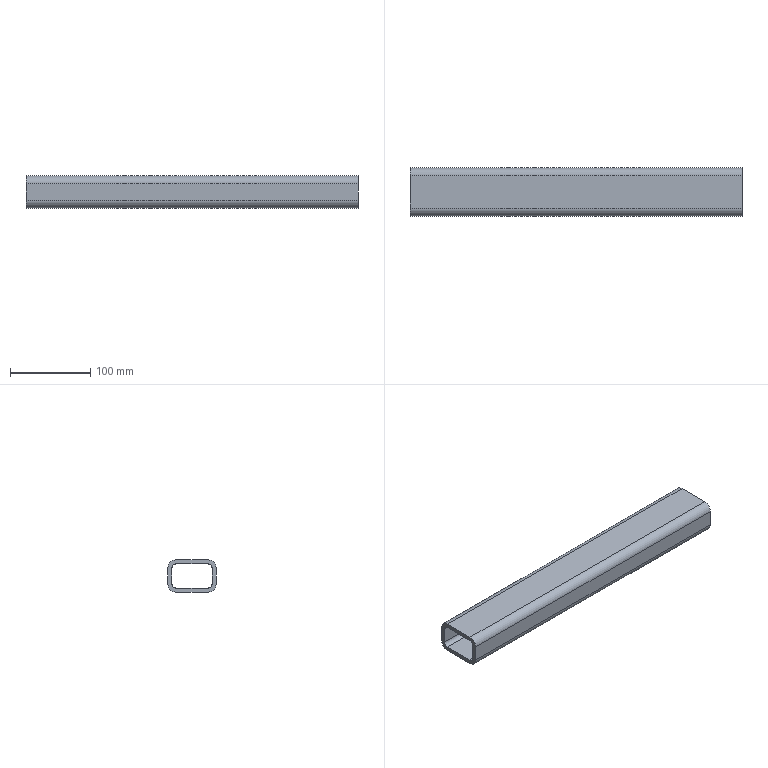Part | STEP file | HL4GD-1.30.112 base frame support longitudinal beam--20251212 | 1 solid | 18 faces | box 414 x 60 x 40 mm | volume 345946 mm3 | plane 10 | cylinder 8 | commonest cylinder face diameters 10 x4 20 x4
STEP:
#1=CARTESIAN_POINT('',(0.,0.,0.));
#2=DIRECTION('',(0.,0.,1.));
#3=DIRECTION('',(1.,0.,0.));
#4=AXIS2_PLACEMENT_3D('',#1,#2,#3);
#5=CARTESIAN_POINT('',(2009.,540.,400.));
#6=VERTEX_POINT('',#5);
#7=CARTESIAN_POINT('',(2009.,535.,395.));
#8=VERTEX_POINT('',#7);
#9=CARTESIAN_POINT('',(2009.,540.,395.));
#10=DIRECTION('',(1.,0.,0.));
#11=DIRECTION('',(0.,0.,-1.));
#12=AXIS2_PLACEMENT_3D('',#9,#10,#11);
#13=CIRCLE('',#12,5.);
#14=CARTESIAN_POINT('',(2555.,540.,395.));
#15=DIRECTION('',(1.,0.,0.));
#16=DIRECTION('',(0.,0.,1.));
#17=AXIS2_PLACEMENT_3D('',#14,#15,#16);
#18=CYLINDRICAL_SURFACE('',#17,5.);
#19=CARTESIAN_POINT('',(-3.142,-546.));
#20=DIRECTION('',(1.,0.));
#21=VECTOR('',#20,1.);
#22=LINE('',#19,#21);
#23=(GEOMETRIC_REPRESENTATION_CONTEXT(2)PARAMETRIC_REPRESENTATION_CONTEXT()REPRESENTATION_CONTEXT('',''));
#24=DEFINITIONAL_REPRESENTATION('',(#22),#23);
#25=PCURVE('',#18,#24);
#26=CARTESIAN_POINT('',(2009.,590.,375.));
#27=DIRECTION('',(1.,0.,0.));
#28=DIRECTION('',(0.,0.,-1.));
#29=AXIS2_PLACEMENT_3D('',#26,#27,#28);
#30=PLANE('',#29);
#31=CARTESIAN_POINT('',(-20.,-50.));
#32=DIRECTION('',(1.,0.));
#33=AXIS2_PLACEMENT_2D('',#31,#32);
#34=CIRCLE('',#33,5.);
#35=(GEOMETRIC_REPRESENTATION_CONTEXT(2)PARAMETRIC_REPRESENTATION_CONTEXT()REPRESENTATION_CONTEXT('',''));
#36=DEFINITIONAL_REPRESENTATION('',(#34),#35);
#37=PCURVE('',#30,#36);
#38=SURFACE_CURVE('',#13,(#25,#37),.PCURVE_S1.);
#39=EDGE_CURVE('',#6,#8,#38,.T.);
#40=ORIENTED_EDGE('',*,*,#39,.F.);
#41=CARTESIAN_POINT('',(1595.,540.,400.));
#42=VERTEX_POINT('',#41);
#43=CARTESIAN_POINT('',(2555.,540.,400.));
#44=DIRECTION('',(-1.,0.,0.));
#45=VECTOR('',#44,1.);
#46=LINE('',#43,#45);
#47=CARTESIAN_POINT('',(0.,0.));
#48=DIRECTION('',(0.,-1.));
#49=VECTOR('',#48,1.);
#50=LINE('',#47,#49);
#51=(GEOMETRIC_REPRESENTATION_CONTEXT(2)PARAMETRIC_REPRESENTATION_CONTEXT()REPRESENTATION_CONTEXT('',''));
#52=DEFINITIONAL_REPRESENTATION('',(#50),#51);
#53=PCURVE('',#18,#52);
#54=CARTESIAN_POINT('',(2555.,540.,400.));
#55=DIRECTION('',(0.,0.,-1.));
#56=DIRECTION('',(0.,-1.,0.));
#57=AXIS2_PLACEMENT_3D('',#54,#55,#56);
#58=PLANE('',#57);
#59=CARTESIAN_POINT('',(0.,0.));
#60=DIRECTION('',(0.,1.));
#61=VECTOR('',#60,1.);
#62=LINE('',#59,#61);
#63=(GEOMETRIC_REPRESENTATION_CONTEXT(2)PARAMETRIC_REPRESENTATION_CONTEXT()REPRESENTATION_CONTEXT('',''));
#64=DEFINITIONAL_REPRESENTATION('',(#62),#63);
#65=PCURVE('',#58,#64);
#66=SURFACE_CURVE('',#46,(#53,#65),.PCURVE_S1.);
#67=EDGE_CURVE('',#6,#42,#66,.T.);
#68=ORIENTED_EDGE('',*,*,#67,.T.);
#69=CARTESIAN_POINT('',(1595.,535.,395.));
#70=VERTEX_POINT('',#69);
#71=CARTESIAN_POINT('',(1595.,540.,395.));
#72=DIRECTION('',(1.,0.,0.));
#73=DIRECTION('',(0.,0.,1.));
#74=AXIS2_PLACEMENT_3D('',#71,#72,#73);
#75=CIRCLE('',#74,5.);
#76=CARTESIAN_POINT('',(0.,-960.));
#77=DIRECTION('',(1.,0.));
#78=VECTOR('',#77,1.);
#79=LINE('',#76,#78);
#80=(GEOMETRIC_REPRESENTATION_CONTEXT(2)PARAMETRIC_REPRESENTATION_CONTEXT()REPRESENTATION_CONTEXT('',''));
#81=DEFINITIONAL_REPRESENTATION('',(#79),#80);
#82=PCURVE('',#18,#81);
#83=CARTESIAN_POINT('',(1595.,406.07,581.07));
#84=DIRECTION('',(1.,0.,0.));
#85=DIRECTION('',(0.,0.,1.));
#86=AXIS2_PLACEMENT_3D('',#83,#84,#85);
#87=PLANE('',#86);
#88=CARTESIAN_POINT('',(-186.07,-133.93));
#89=DIRECTION('',(1.,0.));
#90=AXIS2_PLACEMENT_2D('',#88,#89);
#91=CIRCLE('',#90,5.);
#92=(GEOMETRIC_REPRESENTATION_CONTEXT(2)PARAMETRIC_REPRESENTATION_CONTEXT()REPRESENTATION_CONTEXT('',''));
#93=DEFINITIONAL_REPRESENTATION('',(#91),#92);
#94=PCURVE('',#87,#93);
#95=SURFACE_CURVE('',#75,(#82,#94),.PCURVE_S1.);
#96=EDGE_CURVE('',#42,#70,#95,.T.);
#97=ORIENTED_EDGE('',*,*,#96,.T.);
#98=CARTESIAN_POINT('',(2555.,535.,395.));
#99=DIRECTION('',(-1.,0.,0.));
#100=VECTOR('',#99,1.);
#101=LINE('',#98,#100);
#102=CARTESIAN_POINT('',(1.571,0.));
#103=DIRECTION('',(0.,-1.));
#104=VECTOR('',#103,1.);
#105=LINE('',#102,#104);
#106=(GEOMETRIC_REPRESENTATION_CONTEXT(2)PARAMETRIC_REPRESENTATION_CONTEXT()REPRESENTATION_CONTEXT('',''));
#107=DEFINITIONAL_REPRESENTATION('',(#105),#106);
#108=PCURVE('',#18,#107);
#109=CARTESIAN_POINT('',(2555.,535.,375.));
#110=DIRECTION('',(0.,1.,0.));
#111=DIRECTION('',(0.,0.,-1.));
#112=AXIS2_PLACEMENT_3D('',#109,#110,#111);
#113=PLANE('',#112);
#114=CARTESIAN_POINT('',(-20.,0.));
#115=DIRECTION('',(0.,1.));
#116=VECTOR('',#115,1.);
#117=LINE('',#114,#116);
#118=(GEOMETRIC_REPRESENTATION_CONTEXT(2)PARAMETRIC_REPRESENTATION_CONTEXT()REPRESENTATION_CONTEXT('',''));
#119=DEFINITIONAL_REPRESENTATION('',(#117),#118);
#120=PCURVE('',#113,#119);
#121=SURFACE_CURVE('',#101,(#108,#120),.PCURVE_S1.);
#122=EDGE_CURVE('',#8,#70,#121,.T.);
#123=ORIENTED_EDGE('',*,*,#122,.F.);
#124=EDGE_LOOP('',(#40,#68,#97,#123));
#125=FACE_BOUND('',#124,.F.);
#126=ADVANCED_FACE('',(#125),#18,.F.);
#127=CARTESIAN_POINT('',(2009.,535.,375.));
#128=VERTEX_POINT('',#127);
#129=CARTESIAN_POINT('',(1595.,535.,375.));
#130=VERTEX_POINT('',#129);
#131=CARTESIAN_POINT('',(2555.,535.,375.));
#132=DIRECTION('',(-1.,0.,0.));
#133=VECTOR('',#132,1.);
#134=LINE('',#131,#133);
#135=CARTESIAN_POINT('',(0.,0.));
#136=DIRECTION('',(0.,1.));
#137=VECTOR('',#136,1.);
#138=LINE('',#135,#137);
#139=(GEOMETRIC_REPRESENTATION_CONTEXT(2)PARAMETRIC_REPRESENTATION_CONTEXT()REPRESENTATION_CONTEXT('',''));
#140=DEFINITIONAL_REPRESENTATION('',(#138),#139);
#141=PCURVE('',#113,#140);
#142=CARTESIAN_POINT('',(2555.,540.,375.));
#143=DIRECTION('',(1.,0.,0.));
#144=DIRECTION('',(0.,0.,1.));
#145=AXIS2_PLACEMENT_3D('',#142,#143,#144);
#146=CYLINDRICAL_SURFACE('',#145,5.);
#147=CARTESIAN_POINT('',(1.571,0.));
#148=DIRECTION('',(0.,-1.));
#149=VECTOR('',#148,1.);
#150=LINE('',#147,#149);
#151=(GEOMETRIC_REPRESENTATION_CONTEXT(2)PARAMETRIC_REPRESENTATION_CONTEXT()REPRESENTATION_CONTEXT('',''));
#152=DEFINITIONAL_REPRESENTATION('',(#150),#151);
#153=PCURVE('',#146,#152);
#154=SURFACE_CURVE('',#134,(#141,#153),.PCURVE_S1.);
#155=EDGE_CURVE('',#128,#130,#154,.T.);
#156=ORIENTED_EDGE('',*,*,#155,.T.);
#157=CARTESIAN_POINT('',(1595.,535.,375.));
#158=DIRECTION('',(0.,0.,1.));
#159=VECTOR('',#158,1.);
#160=LINE('',#157,#159);
#161=CARTESIAN_POINT('',(0.,960.));
#162=DIRECTION('',(-1.,0.));
#163=VECTOR('',#162,1.);
#164=LINE('',#161,#163);
#165=(GEOMETRIC_REPRESENTATION_CONTEXT(2)PARAMETRIC_REPRESENTATION_CONTEXT()REPRESENTATION_CONTEXT('',''));
#166=DEFINITIONAL_REPRESENTATION('',(#164),#165);
#167=PCURVE('',#113,#166);
#168=CARTESIAN_POINT('',(-206.07,-128.93));
#169=DIRECTION('',(1.,0.));
#170=VECTOR('',#169,1.);
#171=LINE('',#168,#170);
#172=(GEOMETRIC_REPRESENTATION_CONTEXT(2)PARAMETRIC_REPRESENTATION_CONTEXT()REPRESENTATION_CONTEXT('',''));
#173=DEFINITIONAL_REPRESENTATION('',(#171),#172);
#174=PCURVE('',#87,#173);
#175=SURFACE_CURVE('',#160,(#167,#174),.PCURVE_S1.);
#176=EDGE_CURVE('',#130,#70,#175,.T.);
#177=ORIENTED_EDGE('',*,*,#176,.T.);
#178=ORIENTED_EDGE('',*,*,#122,.F.);
#179=CARTESIAN_POINT('',(2009.,535.,375.));
#180=DIRECTION('',(0.,0.,-1.));
#181=VECTOR('',#180,1.);
#182=LINE('',#179,#181);
#183=CARTESIAN_POINT('',(0.,546.));
#184=DIRECTION('',(1.,0.));
#185=VECTOR('',#184,1.);
#186=LINE('',#183,#185);
#187=(GEOMETRIC_REPRESENTATION_CONTEXT(2)PARAMETRIC_REPRESENTATION_CONTEXT()REPRESENTATION_CONTEXT('',''));
#188=DEFINITIONAL_REPRESENTATION('',(#186),#187);
#189=PCURVE('',#113,#188);
#190=CARTESIAN_POINT('',(0.,-55.));
#191=DIRECTION('',(1.,0.));
#192=VECTOR('',#191,1.);
#193=LINE('',#190,#192);
#194=(GEOMETRIC_REPRESENTATION_CONTEXT(2)PARAMETRIC_REPRESENTATION_CONTEXT()REPRESENTATION_CONTEXT('',''));
#195=DEFINITIONAL_REPRESENTATION('',(#193),#194);
#196=PCURVE('',#30,#195);
#197=SURFACE_CURVE('',#182,(#189,#196),.PCURVE_S1.);
#198=EDGE_CURVE('',#8,#128,#197,.T.);
#199=ORIENTED_EDGE('',*,*,#198,.T.);
#200=EDGE_LOOP('',(#156,#177,#178,#199));
#201=FACE_BOUND('',#200,.T.);
#202=ADVANCED_FACE('',(#201),#113,.T.);
#203=CARTESIAN_POINT('',(2009.,540.,370.));
#204=VERTEX_POINT('',#203);
#205=CARTESIAN_POINT('',(2009.,540.,375.));
#206=DIRECTION('',(1.,0.,0.));
#207=DIRECTION('',(0.,0.,-1.));
#208=AXIS2_PLACEMENT_3D('',#205,#206,#207);
#209=CIRCLE('',#208,5.);
#210=CARTESIAN_POINT('',(-3.142,-546.));
#211=DIRECTION('',(1.,0.));
#212=VECTOR('',#211,1.);
#213=LINE('',#210,#212);
#214=(GEOMETRIC_REPRESENTATION_CONTEXT(2)PARAMETRIC_REPRESENTATION_CONTEXT()REPRESENTATION_CONTEXT('',''));
#215=DEFINITIONAL_REPRESENTATION('',(#213),#214);
#216=PCURVE('',#146,#215);
#217=CARTESIAN_POINT('',(0.,-50.));
#218=DIRECTION('',(1.,0.));
#219=AXIS2_PLACEMENT_2D('',#217,#218);
#220=CIRCLE('',#219,5.);
#221=(GEOMETRIC_REPRESENTATION_CONTEXT(2)PARAMETRIC_REPRESENTATION_CONTEXT()REPRESENTATION_CONTEXT('',''));
#222=DEFINITIONAL_REPRESENTATION('',(#220),#221);
#223=PCURVE('',#30,#222);
#224=SURFACE_CURVE('',#209,(#216,#223),.PCURVE_S1.);
#225=EDGE_CURVE('',#128,#204,#224,.T.);
#226=ORIENTED_EDGE('',*,*,#225,.F.);
#227=ORIENTED_EDGE('',*,*,#155,.T.);
#228=CARTESIAN_POINT('',(1595.,540.,370.));
#229=VERTEX_POINT('',#228);
#230=CARTESIAN_POINT('',(1595.,540.,375.));
#231=DIRECTION('',(-1.,0.,0.));
#232=DIRECTION('',(0.,0.,1.));
#233=AXIS2_PLACEMENT_3D('',#230,#231,#232);
#234=CIRCLE('',#233,5.);
#235=CARTESIAN_POINT('',(6.283,-960.));
#236=DIRECTION('',(-1.,0.));
#237=VECTOR('',#236,1.);
#238=LINE('',#235,#237);
#239=(GEOMETRIC_REPRESENTATION_CONTEXT(2)PARAMETRIC_REPRESENTATION_CONTEXT()REPRESENTATION_CONTEXT('',''));
#240=DEFINITIONAL_REPRESENTATION('',(#238),#239);
#241=PCURVE('',#146,#240);
#242=CARTESIAN_POINT('',(-201.07,-133.93));
#243=CARTESIAN_POINT('',(-201.07,-142.591));
#244=CARTESIAN_POINT('',(-208.57,-138.261));
#245=CARTESIAN_POINT('',(-216.07,-133.93));
#246=CARTESIAN_POINT('',(-208.57,-129.6));
#247=CARTESIAN_POINT('',(-201.07,-125.27));
#248=CARTESIAN_POINT('',(-201.07,-133.93));
#249=(BOUNDED_CURVE()B_SPLINE_CURVE(2,(#242,#243,#244,#245,#246,#247,#248),.UNSPECIFIED.,.T.,.F.)B_SPLINE_CURVE_WITH_KNOTS((1,2,2,2,2,1),(-2.094,0.,2.094,4.189,6.283,8.378),.UNSPECIFIED.)CURVE()GEOMETRIC_REPRESENTATION_ITEM()RATIONAL_B_SPLINE_CURVE((1.,0.5,1.,0.5,1.,0.5,1.))REPRESENTATION_ITEM(''));
#250=(GEOMETRIC_REPRESENTATION_CONTEXT(2)PARAMETRIC_REPRESENTATION_CONTEXT()REPRESENTATION_CONTEXT('',''));
#251=DEFINITIONAL_REPRESENTATION('',(#249),#250);
#252=PCURVE('',#87,#251);
#253=SURFACE_CURVE('',#234,(#241,#252),.PCURVE_S1.);
#254=EDGE_CURVE('',#229,#130,#253,.T.);
#255=ORIENTED_EDGE('',*,*,#254,.F.);
#256=CARTESIAN_POINT('',(2555.,540.,370.));
#257=DIRECTION('',(-1.,0.,0.));
#258=VECTOR('',#257,1.);
#259=LINE('',#256,#258);
#260=CARTESIAN_POINT('',(3.142,0.));
#261=DIRECTION('',(0.,-1.));
#262=VECTOR('',#261,1.);
#263=LINE('',#260,#262);
#264=(GEOMETRIC_REPRESENTATION_CONTEXT(2)PARAMETRIC_REPRESENTATION_CONTEXT()REPRESENTATION_CONTEXT('',''));
#265=DEFINITIONAL_REPRESENTATION('',(#263),#264);
#266=PCURVE('',#146,#265);
#267=CARTESIAN_POINT('',(2555.,580.,370.));
#268=DIRECTION('',(0.,0.,1.));
#269=DIRECTION('',(0.,1.,0.));
#270=AXIS2_PLACEMENT_3D('',#267,#268,#269);
#271=PLANE('',#270);
#272=CARTESIAN_POINT('',(-40.,0.));
#273=DIRECTION('',(0.,1.));
#274=VECTOR('',#273,1.);
#275=LINE('',#272,#274);
#276=(GEOMETRIC_REPRESENTATION_CONTEXT(2)PARAMETRIC_REPRESENTATION_CONTEXT()REPRESENTATION_CONTEXT('',''));
#277=DEFINITIONAL_REPRESENTATION('',(#275),#276);
#278=PCURVE('',#271,#277);
#279=SURFACE_CURVE('',#259,(#266,#278),.PCURVE_S1.);
#280=EDGE_CURVE('',#204,#229,#279,.T.);
#281=ORIENTED_EDGE('',*,*,#280,.F.);
#282=EDGE_LOOP('',(#226,#227,#255,#281));
#283=FACE_BOUND('',#282,.F.);
#284=ADVANCED_FACE('',(#283),#146,.F.);
#285=CARTESIAN_POINT('',(2009.,580.,370.));
#286=VERTEX_POINT('',#285);
#287=CARTESIAN_POINT('',(1595.,580.,370.));
#288=VERTEX_POINT('',#287);
#289=CARTESIAN_POINT('',(2555.,580.,370.));
#290=DIRECTION('',(-1.,0.,0.));
#291=VECTOR('',#290,1.);
#292=LINE('',#289,#291);
#293=CARTESIAN_POINT('',(0.,0.));
#294=DIRECTION('',(0.,1.));
#295=VECTOR('',#294,1.);
#296=LINE('',#293,#295);
#297=(GEOMETRIC_REPRESENTATION_CONTEXT(2)PARAMETRIC_REPRESENTATION_CONTEXT()REPRESENTATION_CONTEXT('',''));
#298=DEFINITIONAL_REPRESENTATION('',(#296),#297);
#299=PCURVE('',#271,#298);
#300=CARTESIAN_POINT('',(2555.,580.,375.));
#301=DIRECTION('',(1.,0.,0.));
#302=DIRECTION('',(0.,0.,1.));
#303=AXIS2_PLACEMENT_3D('',#300,#301,#302);
#304=CYLINDRICAL_SURFACE('',#303,5.);
#305=CARTESIAN_POINT('',(3.142,0.));
#306=DIRECTION('',(0.,-1.));
#307=VECTOR('',#306,1.);
#308=LINE('',#305,#307);
#309=(GEOMETRIC_REPRESENTATION_CONTEXT(2)PARAMETRIC_REPRESENTATION_CONTEXT()REPRESENTATION_CONTEXT('',''));
#310=DEFINITIONAL_REPRESENTATION('',(#308),#309);
#311=PCURVE('',#304,#310);
#312=SURFACE_CURVE('',#292,(#299,#311),.PCURVE_S1.);
#313=EDGE_CURVE('',#286,#288,#312,.T.);
#314=ORIENTED_EDGE('',*,*,#313,.T.);
#315=CARTESIAN_POINT('',(1595.,580.,370.));
#316=DIRECTION('',(0.,1.,0.));
#317=VECTOR('',#316,1.);
#318=LINE('',#315,#317);
#319=CARTESIAN_POINT('',(0.,960.));
#320=DIRECTION('',(1.,0.));
#321=VECTOR('',#320,1.);
#322=LINE('',#319,#321);
#323=(GEOMETRIC_REPRESENTATION_CONTEXT(2)PARAMETRIC_REPRESENTATION_CONTEXT()REPRESENTATION_CONTEXT('',''));
#324=DEFINITIONAL_REPRESENTATION('',(#322),#323);
#325=PCURVE('',#271,#324);
#326=CARTESIAN_POINT('',(-211.07,-173.93));
#327=DIRECTION('',(0.,-1.));
#328=VECTOR('',#327,1.);
#329=LINE('',#326,#328);
#330=(GEOMETRIC_REPRESENTATION_CONTEXT(2)PARAMETRIC_REPRESENTATION_CONTEXT()REPRESENTATION_CONTEXT('',''));
#331=DEFINITIONAL_REPRESENTATION('',(#329),#330);
#332=PCURVE('',#87,#331);
#333=SURFACE_CURVE('',#318,(#325,#332),.PCURVE_S1.);
#334=EDGE_CURVE('',#229,#288,#333,.T.);
#335=ORIENTED_EDGE('',*,*,#334,.F.);
#336=ORIENTED_EDGE('',*,*,#280,.F.);
#337=CARTESIAN_POINT('',(2009.,580.,370.));
#338=DIRECTION('',(0.,1.,0.));
#339=VECTOR('',#338,1.);
#340=LINE('',#337,#339);
#341=CARTESIAN_POINT('',(0.,546.));
#342=DIRECTION('',(1.,0.));
#343=VECTOR('',#342,1.);
#344=LINE('',#341,#343);
#345=(GEOMETRIC_REPRESENTATION_CONTEXT(2)PARAMETRIC_REPRESENTATION_CONTEXT()REPRESENTATION_CONTEXT('',''));
#346=DEFINITIONAL_REPRESENTATION('',(#344),#345);
#347=PCURVE('',#271,#346);
#348=CARTESIAN_POINT('',(5.,-10.));
#349=DIRECTION('',(0.,1.));
#350=VECTOR('',#349,1.);
#351=LINE('',#348,#350);
#352=(GEOMETRIC_REPRESENTATION_CONTEXT(2)PARAMETRIC_REPRESENTATION_CONTEXT()REPRESENTATION_CONTEXT('',''));
#353=DEFINITIONAL_REPRESENTATION('',(#351),#352);
#354=PCURVE('',#30,#353);
#355=SURFACE_CURVE('',#340,(#347,#354),.PCURVE_S1.);
#356=EDGE_CURVE('',#204,#286,#355,.T.);
#357=ORIENTED_EDGE('',*,*,#356,.T.);
#358=EDGE_LOOP('',(#314,#335,#336,#357));
#359=FACE_BOUND('',#358,.T.);
#360=ADVANCED_FACE('',(#359),#271,.T.);
#361=CARTESIAN_POINT('',(2009.,585.,375.));
#362=VERTEX_POINT('',#361);
#363=CARTESIAN_POINT('',(2009.,580.,375.));
#364=DIRECTION('',(1.,0.,0.));
#365=DIRECTION('',(0.,0.,-1.));
#366=AXIS2_PLACEMENT_3D('',#363,#364,#365);
#367=CIRCLE('',#366,5.);
#368=CARTESIAN_POINT('',(3.142,-546.));
#369=DIRECTION('',(1.,0.));
#370=VECTOR('',#369,1.);
#371=LINE('',#368,#370);
#372=(GEOMETRIC_REPRESENTATION_CONTEXT(2)PARAMETRIC_REPRESENTATION_CONTEXT()REPRESENTATION_CONTEXT('',''));
#373=DEFINITIONAL_REPRESENTATION('',(#371),#372);
#374=PCURVE('',#304,#373);
#375=CARTESIAN_POINT('',(0.,-10.));
#376=DIRECTION('',(1.,0.));
#377=AXIS2_PLACEMENT_2D('',#375,#376);
#378=CIRCLE('',#377,5.);
#379=(GEOMETRIC_REPRESENTATION_CONTEXT(2)PARAMETRIC_REPRESENTATION_CONTEXT()REPRESENTATION_CONTEXT('',''));
#380=DEFINITIONAL_REPRESENTATION('',(#378),#379);
#381=PCURVE('',#30,#380);
#382=SURFACE_CURVE('',#367,(#374,#381),.PCURVE_S1.);
#383=EDGE_CURVE('',#286,#362,#382,.T.);
#384=ORIENTED_EDGE('',*,*,#383,.F.);
#385=ORIENTED_EDGE('',*,*,#313,.T.);
#386=CARTESIAN_POINT('',(1595.,585.,375.));
#387=VERTEX_POINT('',#386);
#388=CARTESIAN_POINT('',(1595.,580.,375.));
#389=DIRECTION('',(1.,0.,0.));
#390=DIRECTION('',(0.,0.,1.));
#391=AXIS2_PLACEMENT_3D('',#388,#389,#390);
#392=CIRCLE('',#391,5.);
#393=CARTESIAN_POINT('',(0.,-960.));
#394=DIRECTION('',(1.,0.));
#395=VECTOR('',#394,1.);
#396=LINE('',#393,#395);
#397=(GEOMETRIC_REPRESENTATION_CONTEXT(2)PARAMETRIC_REPRESENTATION_CONTEXT()REPRESENTATION_CONTEXT('',''));
#398=DEFINITIONAL_REPRESENTATION('',(#396),#397);
#399=PCURVE('',#304,#398);
#400=CARTESIAN_POINT('',(-206.07,-173.93));
#401=DIRECTION('',(1.,0.));
#402=AXIS2_PLACEMENT_2D('',#400,#401);
#403=CIRCLE('',#402,5.);
#404=(GEOMETRIC_REPRESENTATION_CONTEXT(2)PARAMETRIC_REPRESENTATION_CONTEXT()REPRESENTATION_CONTEXT('',''));
#405=DEFINITIONAL_REPRESENTATION('',(#403),#404);
#406=PCURVE('',#87,#405);
#407=SURFACE_CURVE('',#392,(#399,#406),.PCURVE_S1.);
#408=EDGE_CURVE('',#288,#387,#407,.T.);
#409=ORIENTED_EDGE('',*,*,#408,.T.);
#410=CARTESIAN_POINT('',(2555.,585.,375.));
#411=DIRECTION('',(-1.,0.,0.));
#412=VECTOR('',#411,1.);
#413=LINE('',#410,#412);
#414=CARTESIAN_POINT('',(4.712,0.));
#415=DIRECTION('',(0.,-1.));
#416=VECTOR('',#415,1.);
#417=LINE('',#414,#416);
#418=(GEOMETRIC_REPRESENTATION_CONTEXT(2)PARAMETRIC_REPRESENTATION_CONTEXT()REPRESENTATION_CONTEXT('',''));
#419=DEFINITIONAL_REPRESENTATION('',(#417),#418);
#420=PCURVE('',#304,#419);
#421=CARTESIAN_POINT('',(2555.,585.,395.));
#422=DIRECTION('',(0.,-1.,0.));
#423=DIRECTION('',(0.,0.,1.));
#424=AXIS2_PLACEMENT_3D('',#421,#422,#423);
#425=PLANE('',#424);
#426=CARTESIAN_POINT('',(-20.,0.));
#427=DIRECTION('',(0.,1.));
#428=VECTOR('',#427,1.);
#429=LINE('',#426,#428);
#430=(GEOMETRIC_REPRESENTATION_CONTEXT(2)PARAMETRIC_REPRESENTATION_CONTEXT()REPRESENTATION_CONTEXT('',''));
#431=DEFINITIONAL_REPRESENTATION('',(#429),#430);
#432=PCURVE('',#425,#431);
#433=SURFACE_CURVE('',#413,(#420,#432),.PCURVE_S1.);
#434=EDGE_CURVE('',#362,#387,#433,.T.);
#435=ORIENTED_EDGE('',*,*,#434,.F.);
#436=EDGE_LOOP('',(#384,#385,#409,#435));
#437=FACE_BOUND('',#436,.F.);
#438=ADVANCED_FACE('',(#437),#304,.F.);
#439=CARTESIAN_POINT('',(2009.,585.,395.));
#440=VERTEX_POINT('',#439);
#441=CARTESIAN_POINT('',(1595.,585.,395.));
#442=VERTEX_POINT('',#441);
#443=CARTESIAN_POINT('',(2555.,585.,395.));
#444=DIRECTION('',(-1.,0.,0.));
#445=VECTOR('',#444,1.);
#446=LINE('',#443,#445);
#447=CARTESIAN_POINT('',(0.,0.));
#448=DIRECTION('',(0.,1.));
#449=VECTOR('',#448,1.);
#450=LINE('',#447,#449);
#451=(GEOMETRIC_REPRESENTATION_CONTEXT(2)PARAMETRIC_REPRESENTATION_CONTEXT()REPRESENTATION_CONTEXT('',''));
#452=DEFINITIONAL_REPRESENTATION('',(#450),#451);
#453=PCURVE('',#425,#452);
#454=CARTESIAN_POINT('',(2555.,580.,395.));
#455=DIRECTION('',(1.,0.,0.));
#456=DIRECTION('',(0.,0.,1.));
#457=AXIS2_PLACEMENT_3D('',#454,#455,#456);
#458=CYLINDRICAL_SURFACE('',#457,5.);
#459=CARTESIAN_POINT('',(4.712,0.));
#460=DIRECTION('',(0.,-1.));
#461=VECTOR('',#460,1.);
#462=LINE('',#459,#461);
#463=(GEOMETRIC_REPRESENTATION_CONTEXT(2)PARAMETRIC_REPRESENTATION_CONTEXT()REPRESENTATION_CONTEXT('',''));
#464=DEFINITIONAL_REPRESENTATION('',(#462),#463);
#465=PCURVE('',#458,#464);
#466=SURFACE_CURVE('',#446,(#453,#465),.PCURVE_S1.);
#467=EDGE_CURVE('',#440,#442,#466,.T.);
#468=ORIENTED_EDGE('',*,*,#467,.T.);
#469=CARTESIAN_POINT('',(1595.,585.,395.));
#470=DIRECTION('',(0.,0.,1.));
#471=VECTOR('',#470,1.);
#472=LINE('',#469,#471);
#473=CARTESIAN_POINT('',(0.,960.));
#474=DIRECTION('',(1.,0.));
#475=VECTOR('',#474,1.);
#476=LINE('',#473,#475);
#477=(GEOMETRIC_REPRESENTATION_CONTEXT(2)PARAMETRIC_REPRESENTATION_CONTEXT()REPRESENTATION_CONTEXT('',''));
#478=DEFINITIONAL_REPRESENTATION('',(#476),#477);
#479=PCURVE('',#425,#478);
#480=CARTESIAN_POINT('',(-186.07,-178.93));
#481=DIRECTION('',(1.,0.));
#482=VECTOR('',#481,1.);
#483=LINE('',#480,#482);
#484=(GEOMETRIC_REPRESENTATION_CONTEXT(2)PARAMETRIC_REPRESENTATION_CONTEXT()REPRESENTATION_CONTEXT('',''));
#485=DEFINITIONAL_REPRESENTATION('',(#483),#484);
#486=PCURVE('',#87,#485);
#487=SURFACE_CURVE('',#472,(#479,#486),.PCURVE_S1.);
#488=EDGE_CURVE('',#387,#442,#487,.T.);
#489=ORIENTED_EDGE('',*,*,#488,.F.);
#490=ORIENTED_EDGE('',*,*,#434,.F.);
#491=CARTESIAN_POINT('',(2009.,585.,395.));
#492=DIRECTION('',(0.,0.,1.));
#493=VECTOR('',#492,1.);
#494=LINE('',#491,#493);
#495=CARTESIAN_POINT('',(0.,546.));
#496=DIRECTION('',(1.,0.));
#497=VECTOR('',#496,1.);
#498=LINE('',#495,#497);
#499=(GEOMETRIC_REPRESENTATION_CONTEXT(2)PARAMETRIC_REPRESENTATION_CONTEXT()REPRESENTATION_CONTEXT('',''));
#500=DEFINITIONAL_REPRESENTATION('',(#498),#499);
#501=PCURVE('',#425,#500);
#502=CARTESIAN_POINT('',(-20.,-5.));
#503=DIRECTION('',(-1.,0.));
#504=VECTOR('',#503,1.);
#505=LINE('',#502,#504);
#506=(GEOMETRIC_REPRESENTATION_CONTEXT(2)PARAMETRIC_REPRESENTATION_CONTEXT()REPRESENTATION_CONTEXT('',''));
#507=DEFINITIONAL_REPRESENTATION('',(#505),#506);
#508=PCURVE('',#30,#507);
#509=SURFACE_CURVE('',#494,(#501,#508),.PCURVE_S1.);
#510=EDGE_CURVE('',#362,#440,#509,.T.);
#511=ORIENTED_EDGE('',*,*,#510,.T.);
#512=EDGE_LOOP('',(#468,#489,#490,#511));
#513=FACE_BOUND('',#512,.T.);
#514=ADVANCED_FACE('',(#513),#425,.T.);
#515=CARTESIAN_POINT('',(2009.,580.,400.));
#516=VERTEX_POINT('',#515);
#517=CARTESIAN_POINT('',(2009.,580.,395.));
#518=DIRECTION('',(1.,0.,0.));
#519=DIRECTION('',(0.,0.,-1.));
#520=AXIS2_PLACEMENT_3D('',#517,#518,#519);
#521=CIRCLE('',#520,5.);
#522=CARTESIAN_POINT('',(3.142,-546.));
#523=DIRECTION('',(1.,0.));
#524=VECTOR('',#523,1.);
#525=LINE('',#522,#524);
#526=(GEOMETRIC_REPRESENTATION_CONTEXT(2)PARAMETRIC_REPRESENTATION_CONTEXT()REPRESENTATION_CONTEXT('',''));
#527=DEFINITIONAL_REPRESENTATION('',(#525),#526);
#528=PCURVE('',#458,#527);
#529=CARTESIAN_POINT('',(-20.,-10.));
#530=DIRECTION('',(1.,0.));
#531=AXIS2_PLACEMENT_2D('',#529,#530);
#532=CIRCLE('',#531,5.);
#533=(GEOMETRIC_REPRESENTATION_CONTEXT(2)PARAMETRIC_REPRESENTATION_CONTEXT()REPRESENTATION_CONTEXT('',''));
#534=DEFINITIONAL_REPRESENTATION('',(#532),#533);
#535=PCURVE('',#30,#534);
#536=SURFACE_CURVE('',#521,(#528,#535),.PCURVE_S1.);
#537=EDGE_CURVE('',#440,#516,#536,.T.);
#538=ORIENTED_EDGE('',*,*,#537,.F.);
#539=ORIENTED_EDGE('',*,*,#467,.T.);
#540=CARTESIAN_POINT('',(1595.,580.,400.));
#541=VERTEX_POINT('',#540);
#542=CARTESIAN_POINT('',(1595.,580.,395.));
#543=DIRECTION('',(-1.,0.,0.));
#544=DIRECTION('',(0.,0.,1.));
#545=AXIS2_PLACEMENT_3D('',#542,#543,#544);
#546=CIRCLE('',#545,5.);
#547=CARTESIAN_POINT('',(6.283,-960.));
#548=DIRECTION('',(-1.,0.));
#549=VECTOR('',#548,1.);
#550=LINE('',#547,#549);
#551=(GEOMETRIC_REPRESENTATION_CONTEXT(2)PARAMETRIC_REPRESENTATION_CONTEXT()REPRESENTATION_CONTEXT('',''));
#552=DEFINITIONAL_REPRESENTATION('',(#550),#551);
#553=PCURVE('',#458,#552);
#554=CARTESIAN_POINT('',(-181.07,-173.93));
#555=CARTESIAN_POINT('',(-181.07,-182.591));
#556=CARTESIAN_POINT('',(-188.57,-178.261));
#557=CARTESIAN_POINT('',(-196.07,-173.93));
#558=CARTESIAN_POINT('',(-188.57,-169.6));
#559=CARTESIAN_POINT('',(-181.07,-165.27));
#560=CARTESIAN_POINT('',(-181.07,-173.93));
#561=(BOUNDED_CURVE()B_SPLINE_CURVE(2,(#554,#555,#556,#557,#558,#559,#560),.UNSPECIFIED.,.T.,.F.)B_SPLINE_CURVE_WITH_KNOTS((1,2,2,2,2,1),(-2.094,0.,2.094,4.189,6.283,8.378),.UNSPECIFIED.)CURVE()GEOMETRIC_REPRESENTATION_ITEM()RATIONAL_B_SPLINE_CURVE((1.,0.5,1.,0.5,1.,0.5,1.))REPRESENTATION_ITEM(''));
#562=(GEOMETRIC_REPRESENTATION_CONTEXT(2)PARAMETRIC_REPRESENTATION_CONTEXT()REPRESENTATION_CONTEXT('',''));
#563=DEFINITIONAL_REPRESENTATION('',(#561),#562);
#564=PCURVE('',#87,#563);
#565=SURFACE_CURVE('',#546,(#553,#564),.PCURVE_S1.);
#566=EDGE_CURVE('',#541,#442,#565,.T.);
#567=ORIENTED_EDGE('',*,*,#566,.F.);
#568=CARTESIAN_POINT('',(2555.,580.,400.));
#569=DIRECTION('',(-1.,0.,0.));
#570=VECTOR('',#569,1.);
#571=LINE('',#568,#570);
#572=CARTESIAN_POINT('',(6.283,0.));
#573=DIRECTION('',(0.,-1.));
#574=VECTOR('',#573,1.);
#575=LINE('',#572,#574);
#576=(GEOMETRIC_REPRESENTATION_CONTEXT(2)PARAMETRIC_REPRESENTATION_CONTEXT()REPRESENTATION_CONTEXT('',''));
#577=DEFINITIONAL_REPRESENTATION('',(#575),#576);
#578=PCURVE('',#458,#577);
#579=CARTESIAN_POINT('',(-40.,0.));
#580=DIRECTION('',(0.,1.));
#581=VECTOR('',#580,1.);
#582=LINE('',#579,#581);
#583=(GEOMETRIC_REPRESENTATION_CONTEXT(2)PARAMETRIC_REPRESENTATION_CONTEXT()REPRESENTATION_CONTEXT('',''));
#584=DEFINITIONAL_REPRESENTATION('',(#582),#583);
#585=PCURVE('',#58,#584);
#586=SURFACE_CURVE('',#571,(#578,#585),.PCURVE_S1.);
#587=EDGE_CURVE('',#516,#541,#586,.T.);
#588=ORIENTED_EDGE('',*,*,#587,.F.);
#589=EDGE_LOOP('',(#538,#539,#567,#588));
#590=FACE_BOUND('',#589,.F.);
#591=ADVANCED_FACE('',(#590),#458,.F.);
#592=CARTESIAN_POINT('',(2009.,540.,365.));
#593=VERTEX_POINT('',#592);
#594=CARTESIAN_POINT('',(1595.,540.,365.));
#595=VERTEX_POINT('',#594);
#596=CARTESIAN_POINT('',(2555.,540.,365.));
#597=DIRECTION('',(-1.,0.,0.));
#598=VECTOR('',#597,1.);
#599=LINE('',#596,#598);
#600=CARTESIAN_POINT('',(2555.,580.,365.));
#601=DIRECTION('',(0.,0.,1.));
#602=DIRECTION('',(0.,1.,0.));
#603=AXIS2_PLACEMENT_3D('',#600,#601,#602);
#604=PLANE('',#603);
#605=CARTESIAN_POINT('',(-40.,0.));
#606=DIRECTION('',(0.,1.));
#607=VECTOR('',#606,1.);
#608=LINE('',#605,#607);
#609=(GEOMETRIC_REPRESENTATION_CONTEXT(2)PARAMETRIC_REPRESENTATION_CONTEXT()REPRESENTATION_CONTEXT('',''));
#610=DEFINITIONAL_REPRESENTATION('',(#608),#609);
#611=PCURVE('',#604,#610);
#612=CARTESIAN_POINT('',(2555.,540.,375.));
#613=DIRECTION('',(1.,0.,0.));
#614=DIRECTION('',(0.,0.,1.));
#615=AXIS2_PLACEMENT_3D('',#612,#613,#614);
#616=CYLINDRICAL_SURFACE('',#615,10.);
#617=CARTESIAN_POINT('',(3.142,0.));
#618=DIRECTION('',(0.,-1.));
#619=VECTOR('',#618,1.);
#620=LINE('',#617,#619);
#621=(GEOMETRIC_REPRESENTATION_CONTEXT(2)PARAMETRIC_REPRESENTATION_CONTEXT()REPRESENTATION_CONTEXT('',''));
#622=DEFINITIONAL_REPRESENTATION('',(#620),#621);
#623=PCURVE('',#616,#622);
#624=SURFACE_CURVE('',#599,(#611,#623),.PCURVE_S1.);
#625=EDGE_CURVE('',#593,#595,#624,.T.);
#626=ORIENTED_EDGE('',*,*,#625,.T.);
#627=CARTESIAN_POINT('',(1595.,580.,365.));
#628=VERTEX_POINT('',#627);
#629=CARTESIAN_POINT('',(1595.,580.,365.));
#630=DIRECTION('',(0.,-1.,0.));
#631=VECTOR('',#630,1.);
#632=LINE('',#629,#631);
#633=CARTESIAN_POINT('',(0.,960.));
#634=DIRECTION('',(-1.,0.));
#635=VECTOR('',#634,1.);
#636=LINE('',#633,#635);
#637=(GEOMETRIC_REPRESENTATION_CONTEXT(2)PARAMETRIC_REPRESENTATION_CONTEXT()REPRESENTATION_CONTEXT('',''));
#638=DEFINITIONAL_REPRESENTATION('',(#636),#637);
#639=PCURVE('',#604,#638);
#640=CARTESIAN_POINT('',(-216.07,-173.93));
#641=DIRECTION('',(0.,1.));
#642=VECTOR('',#641,1.);
#643=LINE('',#640,#642);
#644=(GEOMETRIC_REPRESENTATION_CONTEXT(2)PARAMETRIC_REPRESENTATION_CONTEXT()REPRESENTATION_CONTEXT('',''));
#645=DEFINITIONAL_REPRESENTATION('',(#643),#644);
#646=PCURVE('',#87,#645);
#647=SURFACE_CURVE('',#632,(#639,#646),.PCURVE_S1.);
#648=EDGE_CURVE('',#628,#595,#647,.T.);
#649=ORIENTED_EDGE('',*,*,#648,.F.);
#650=CARTESIAN_POINT('',(2009.,580.,365.));
#651=VERTEX_POINT('',#650);
#652=CARTESIAN_POINT('',(2555.,580.,365.));
#653=DIRECTION('',(-1.,0.,0.));
#654=VECTOR('',#653,1.);
#655=LINE('',#652,#654);
#656=CARTESIAN_POINT('',(0.,0.));
#657=DIRECTION('',(0.,1.));
#658=VECTOR('',#657,1.);
#659=LINE('',#656,#658);
#660=(GEOMETRIC_REPRESENTATION_CONTEXT(2)PARAMETRIC_REPRESENTATION_CONTEXT()REPRESENTATION_CONTEXT('',''));
#661=DEFINITIONAL_REPRESENTATION('',(#659),#660);
#662=PCURVE('',#604,#661);
#663=CARTESIAN_POINT('',(2555.,580.,375.));
#664=DIRECTION('',(1.,0.,0.));
#665=DIRECTION('',(0.,0.,1.));
#666=AXIS2_PLACEMENT_3D('',#663,#664,#665);
#667=CYLINDRICAL_SURFACE('',#666,10.);
#668=CARTESIAN_POINT('',(3.142,0.));
#669=DIRECTION('',(0.,-1.));
#670=VECTOR('',#669,1.);
#671=LINE('',#668,#670);
#672=(GEOMETRIC_REPRESENTATION_CONTEXT(2)PARAMETRIC_REPRESENTATION_CONTEXT()REPRESENTATION_CONTEXT('',''));
#673=DEFINITIONAL_REPRESENTATION('',(#671),#672);
#674=PCURVE('',#667,#673);
#675=SURFACE_CURVE('',#655,(#662,#674),.PCURVE_S1.);
#676=EDGE_CURVE('',#651,#628,#675,.T.);
#677=ORIENTED_EDGE('',*,*,#676,.F.);
#678=CARTESIAN_POINT('',(2009.,580.,365.));
#679=DIRECTION('',(0.,-1.,0.));
#680=VECTOR('',#679,1.);
#681=LINE('',#678,#680);
#682=CARTESIAN_POINT('',(0.,546.));
#683=DIRECTION('',(-1.,0.));
#684=VECTOR('',#683,1.);
#685=LINE('',#682,#684);
#686=(GEOMETRIC_REPRESENTATION_CONTEXT(2)PARAMETRIC_REPRESENTATION_CONTEXT()REPRESENTATION_CONTEXT('',''));
#687=DEFINITIONAL_REPRESENTATION('',(#685),#686);
#688=PCURVE('',#604,#687);
#689=CARTESIAN_POINT('',(10.,-10.));
#690=DIRECTION('',(0.,-1.));
#691=VECTOR('',#690,1.);
#692=LINE('',#689,#691);
#693=(GEOMETRIC_REPRESENTATION_CONTEXT(2)PARAMETRIC_REPRESENTATION_CONTEXT()REPRESENTATION_CONTEXT('',''));
#694=DEFINITIONAL_REPRESENTATION('',(#692),#693);
#695=PCURVE('',#30,#694);
#696=SURFACE_CURVE('',#681,(#688,#695),.PCURVE_S1.);
#697=EDGE_CURVE('',#651,#593,#696,.T.);
#698=ORIENTED_EDGE('',*,*,#697,.T.);
#699=EDGE_LOOP('',(#626,#649,#677,#698));
#700=FACE_BOUND('',#699,.T.);
#701=ADVANCED_FACE('',(#700),#604,.F.);
#702=CARTESIAN_POINT('',(2009.,530.,375.));
#703=VERTEX_POINT('',#702);
#704=CARTESIAN_POINT('',(1595.,530.,375.));
#705=VERTEX_POINT('',#704);
#706=CARTESIAN_POINT('',(2555.,530.,375.));
#707=DIRECTION('',(-1.,0.,0.));
#708=VECTOR('',#707,1.);
#709=LINE('',#706,#708);
#710=CARTESIAN_POINT('',(1.571,0.));
#711=DIRECTION('',(0.,-1.));
#712=VECTOR('',#711,1.);
#713=LINE('',#710,#712);
#714=(GEOMETRIC_REPRESENTATION_CONTEXT(2)PARAMETRIC_REPRESENTATION_CONTEXT()REPRESENTATION_CONTEXT('',''));
#715=DEFINITIONAL_REPRESENTATION('',(#713),#714);
#716=PCURVE('',#616,#715);
#717=CARTESIAN_POINT('',(2555.,530.,375.));
#718=DIRECTION('',(0.,1.,0.));
#719=DIRECTION('',(0.,0.,-1.));
#720=AXIS2_PLACEMENT_3D('',#717,#718,#719);
#721=PLANE('',#720);
#722=CARTESIAN_POINT('',(0.,0.));
#723=DIRECTION('',(0.,1.));
#724=VECTOR('',#723,1.);
#725=LINE('',#722,#724);
#726=(GEOMETRIC_REPRESENTATION_CONTEXT(2)PARAMETRIC_REPRESENTATION_CONTEXT()REPRESENTATION_CONTEXT('',''));
#727=DEFINITIONAL_REPRESENTATION('',(#725),#726);
#728=PCURVE('',#721,#727);
#729=SURFACE_CURVE('',#709,(#716,#728),.PCURVE_S1.);
#730=EDGE_CURVE('',#703,#705,#729,.T.);
#731=ORIENTED_EDGE('',*,*,#730,.T.);
#732=CARTESIAN_POINT('',(1595.,540.,375.));
#733=DIRECTION('',(-1.,0.,0.));
#734=DIRECTION('',(0.,0.,1.));
#735=AXIS2_PLACEMENT_3D('',#732,#733,#734);
#736=CIRCLE('',#735,10.);
#737=CARTESIAN_POINT('',(6.283,-960.));
#738=DIRECTION('',(-1.,0.));
#739=VECTOR('',#738,1.);
#740=LINE('',#737,#739);
#741=(GEOMETRIC_REPRESENTATION_CONTEXT(2)PARAMETRIC_REPRESENTATION_CONTEXT()REPRESENTATION_CONTEXT('',''));
#742=DEFINITIONAL_REPRESENTATION('',(#740),#741);
#743=PCURVE('',#616,#742);
#744=CARTESIAN_POINT('',(-196.07,-133.93));
#745=CARTESIAN_POINT('',(-196.07,-151.251));
#746=CARTESIAN_POINT('',(-211.07,-142.591));
#747=CARTESIAN_POINT('',(-226.07,-133.93));
#748=CARTESIAN_POINT('',(-211.07,-125.27));
#749=CARTESIAN_POINT('',(-196.07,-116.61));
#750=CARTESIAN_POINT('',(-196.07,-133.93));
#751=(BOUNDED_CURVE()B_SPLINE_CURVE(2,(#744,#745,#746,#747,#748,#749,#750),.UNSPECIFIED.,.T.,.F.)B_SPLINE_CURVE_WITH_KNOTS((1,2,2,2,2,1),(-2.094,0.,2.094,4.189,6.283,8.378),.UNSPECIFIED.)CURVE()GEOMETRIC_REPRESENTATION_ITEM()RATIONAL_B_SPLINE_CURVE((1.,0.5,1.,0.5,1.,0.5,1.))REPRESENTATION_ITEM(''));
#752=(GEOMETRIC_REPRESENTATION_CONTEXT(2)PARAMETRIC_REPRESENTATION_CONTEXT()REPRESENTATION_CONTEXT('',''));
#753=DEFINITIONAL_REPRESENTATION('',(#751),#752);
#754=PCURVE('',#87,#753);
#755=SURFACE_CURVE('',#736,(#743,#754),.PCURVE_S1.);
#756=EDGE_CURVE('',#595,#705,#755,.T.);
#757=ORIENTED_EDGE('',*,*,#756,.F.);
#758=ORIENTED_EDGE('',*,*,#625,.F.);
#759=CARTESIAN_POINT('',(2009.,540.,375.));
#760=DIRECTION('',(-1.,0.,0.));
#761=DIRECTION('',(0.,0.,-1.));
#762=AXIS2_PLACEMENT_3D('',#759,#760,#761);
#763=CIRCLE('',#762,10.);
#764=CARTESIAN_POINT('',(3.142,-546.));
#765=DIRECTION('',(-1.,0.));
#766=VECTOR('',#765,1.);
#767=LINE('',#764,#766);
#768=(GEOMETRIC_REPRESENTATION_CONTEXT(2)PARAMETRIC_REPRESENTATION_CONTEXT()REPRESENTATION_CONTEXT('',''));
#769=DEFINITIONAL_REPRESENTATION('',(#767),#768);
#770=PCURVE('',#616,#769);
#771=CARTESIAN_POINT('',(10.,-50.));
#772=CARTESIAN_POINT('',(10.,-67.321));
#773=CARTESIAN_POINT('',(-5.,-58.66));
#774=CARTESIAN_POINT('',(-20.,-50.));
#775=CARTESIAN_POINT('',(-5.,-41.34));
#776=CARTESIAN_POINT('',(10.,-32.679));
#777=CARTESIAN_POINT('',(10.,-50.));
#778=(BOUNDED_CURVE()B_SPLINE_CURVE(2,(#771,#772,#773,#774,#775,#776,#777),.UNSPECIFIED.,.T.,.F.)B_SPLINE_CURVE_WITH_KNOTS((1,2,2,2,2,1),(-2.094,0.,2.094,4.189,6.283,8.378),.UNSPECIFIED.)CURVE()GEOMETRIC_REPRESENTATION_ITEM()RATIONAL_B_SPLINE_CURVE((1.,0.5,1.,0.5,1.,0.5,1.))REPRESENTATION_ITEM(''));
#779=(GEOMETRIC_REPRESENTATION_CONTEXT(2)PARAMETRIC_REPRESENTATION_CONTEXT()REPRESENTATION_CONTEXT('',''));
#780=DEFINITIONAL_REPRESENTATION('',(#778),#779);
#781=PCURVE('',#30,#780);
#782=SURFACE_CURVE('',#763,(#770,#781),.PCURVE_S1.);
#783=EDGE_CURVE('',#593,#703,#782,.T.);
#784=ORIENTED_EDGE('',*,*,#783,.T.);
#785=EDGE_LOOP('',(#731,#757,#758,#784));
#786=FACE_BOUND('',#785,.T.);
#787=ADVANCED_FACE('',(#786),#616,.T.);
#788=CARTESIAN_POINT('',(2009.,530.,395.));
#789=VERTEX_POINT('',#788);
#790=CARTESIAN_POINT('',(1595.,530.,395.));
#791=VERTEX_POINT('',#790);
#792=CARTESIAN_POINT('',(2555.,530.,395.));
#793=DIRECTION('',(-1.,0.,0.));
#794=VECTOR('',#793,1.);
#795=LINE('',#792,#794);
#796=CARTESIAN_POINT('',(-20.,0.));
#797=DIRECTION('',(0.,1.));
#798=VECTOR('',#797,1.);
#799=LINE('',#796,#798);
#800=(GEOMETRIC_REPRESENTATION_CONTEXT(2)PARAMETRIC_REPRESENTATION_CONTEXT()REPRESENTATION_CONTEXT('',''));
#801=DEFINITIONAL_REPRESENTATION('',(#799),#800);
#802=PCURVE('',#721,#801);
#803=CARTESIAN_POINT('',(2555.,540.,395.));
#804=DIRECTION('',(1.,0.,0.));
#805=DIRECTION('',(0.,0.,1.));
#806=AXIS2_PLACEMENT_3D('',#803,#804,#805);
#807=CYLINDRICAL_SURFACE('',#806,10.);
#808=CARTESIAN_POINT('',(1.571,0.));
#809=DIRECTION('',(0.,-1.));
#810=VECTOR('',#809,1.);
#811=LINE('',#808,#810);
#812=(GEOMETRIC_REPRESENTATION_CONTEXT(2)PARAMETRIC_REPRESENTATION_CONTEXT()REPRESENTATION_CONTEXT('',''));
#813=DEFINITIONAL_REPRESENTATION('',(#811),#812);
#814=PCURVE('',#807,#813);
#815=SURFACE_CURVE('',#795,(#802,#814),.PCURVE_S1.);
#816=EDGE_CURVE('',#789,#791,#815,.T.);
#817=ORIENTED_EDGE('',*,*,#816,.T.);
#818=CARTESIAN_POINT('',(1595.,530.,375.));
#819=DIRECTION('',(0.,0.,1.));
#820=VECTOR('',#819,1.);
#821=LINE('',#818,#820);
#822=CARTESIAN_POINT('',(0.,960.));
#823=DIRECTION('',(-1.,0.));
#824=VECTOR('',#823,1.);
#825=LINE('',#822,#824);
#826=(GEOMETRIC_REPRESENTATION_CONTEXT(2)PARAMETRIC_REPRESENTATION_CONTEXT()REPRESENTATION_CONTEXT('',''));
#827=DEFINITIONAL_REPRESENTATION('',(#825),#826);
#828=PCURVE('',#721,#827);
#829=CARTESIAN_POINT('',(-206.07,-123.93));
#830=DIRECTION('',(1.,0.));
#831=VECTOR('',#830,1.);
#832=LINE('',#829,#831);
#833=(GEOMETRIC_REPRESENTATION_CONTEXT(2)PARAMETRIC_REPRESENTATION_CONTEXT()REPRESENTATION_CONTEXT('',''));
#834=DEFINITIONAL_REPRESENTATION('',(#832),#833);
#835=PCURVE('',#87,#834);
#836=SURFACE_CURVE('',#821,(#828,#835),.PCURVE_S1.);
#837=EDGE_CURVE('',#705,#791,#836,.T.);
#838=ORIENTED_EDGE('',*,*,#837,.F.);
#839=ORIENTED_EDGE('',*,*,#730,.F.);
#840=CARTESIAN_POINT('',(2009.,530.,375.));
#841=DIRECTION('',(0.,0.,1.));
#842=VECTOR('',#841,1.);
#843=LINE('',#840,#842);
#844=CARTESIAN_POINT('',(0.,546.));
#845=DIRECTION('',(-1.,0.));
#846=VECTOR('',#845,1.);
#847=LINE('',#844,#846);
#848=(GEOMETRIC_REPRESENTATION_CONTEXT(2)PARAMETRIC_REPRESENTATION_CONTEXT()REPRESENTATION_CONTEXT('',''));
#849=DEFINITIONAL_REPRESENTATION('',(#847),#848);
#850=PCURVE('',#721,#849);
#851=CARTESIAN_POINT('',(0.,-60.));
#852=DIRECTION('',(-1.,0.));
#853=VECTOR('',#852,1.);
#854=LINE('',#851,#853);
#855=(GEOMETRIC_REPRESENTATION_CONTEXT(2)PARAMETRIC_REPRESENTATION_CONTEXT()REPRESENTATION_CONTEXT('',''));
#856=DEFINITIONAL_REPRESENTATION('',(#854),#855);
#857=PCURVE('',#30,#856);
#858=SURFACE_CURVE('',#843,(#850,#857),.PCURVE_S1.);
#859=EDGE_CURVE('',#703,#789,#858,.T.);
#860=ORIENTED_EDGE('',*,*,#859,.T.);
#861=EDGE_LOOP('',(#817,#838,#839,#860));
#862=FACE_BOUND('',#861,.T.);
#863=ADVANCED_FACE('',(#862),#721,.F.);
#864=CARTESIAN_POINT('',(2009.,540.,405.));
#865=VERTEX_POINT('',#864);
#866=CARTESIAN_POINT('',(1595.,540.,405.));
#867=VERTEX_POINT('',#866);
#868=CARTESIAN_POINT('',(2555.,540.,405.));
#869=DIRECTION('',(-1.,0.,0.));
#870=VECTOR('',#869,1.);
#871=LINE('',#868,#870);
#872=CARTESIAN_POINT('',(0.,0.));
#873=DIRECTION('',(0.,-1.));
#874=VECTOR('',#873,1.);
#875=LINE('',#872,#874);
#876=(GEOMETRIC_REPRESENTATION_CONTEXT(2)PARAMETRIC_REPRESENTATION_CONTEXT()REPRESENTATION_CONTEXT('',''));
#877=DEFINITIONAL_REPRESENTATION('',(#875),#876);
#878=PCURVE('',#807,#877);
#879=CARTESIAN_POINT('',(2555.,540.,405.));
#880=DIRECTION('',(0.,0.,-1.));
#881=DIRECTION('',(0.,-1.,0.));
#882=AXIS2_PLACEMENT_3D('',#879,#880,#881);
#883=PLANE('',#882);
#884=CARTESIAN_POINT('',(0.,0.));
#885=DIRECTION('',(0.,1.));
#886=VECTOR('',#885,1.);
#887=LINE('',#884,#886);
#888=(GEOMETRIC_REPRESENTATION_CONTEXT(2)PARAMETRIC_REPRESENTATION_CONTEXT()REPRESENTATION_CONTEXT('',''));
#889=DEFINITIONAL_REPRESENTATION('',(#887),#888);
#890=PCURVE('',#883,#889);
#891=SURFACE_CURVE('',#871,(#878,#890),.PCURVE_S1.);
#892=EDGE_CURVE('',#865,#867,#891,.T.);
#893=ORIENTED_EDGE('',*,*,#892,.T.);
#894=CARTESIAN_POINT('',(1595.,540.,395.));
#895=DIRECTION('',(1.,0.,0.));
#896=DIRECTION('',(0.,0.,1.));
#897=AXIS2_PLACEMENT_3D('',#894,#895,#896);
#898=CIRCLE('',#897,10.);
#899=CARTESIAN_POINT('',(0.,-960.));
#900=DIRECTION('',(1.,0.));
#901=VECTOR('',#900,1.);
#902=LINE('',#899,#901);
#903=(GEOMETRIC_REPRESENTATION_CONTEXT(2)PARAMETRIC_REPRESENTATION_CONTEXT()REPRESENTATION_CONTEXT('',''));
#904=DEFINITIONAL_REPRESENTATION('',(#902),#903);
#905=PCURVE('',#807,#904);
#906=CARTESIAN_POINT('',(-186.07,-133.93));
#907=DIRECTION('',(1.,0.));
#908=AXIS2_PLACEMENT_2D('',#906,#907);
#909=CIRCLE('',#908,10.);
#910=(GEOMETRIC_REPRESENTATION_CONTEXT(2)PARAMETRIC_REPRESENTATION_CONTEXT()REPRESENTATION_CONTEXT('',''));
#911=DEFINITIONAL_REPRESENTATION('',(#909),#910);
#912=PCURVE('',#87,#911);
#913=SURFACE_CURVE('',#898,(#905,#912),.PCURVE_S1.);
#914=EDGE_CURVE('',#867,#791,#913,.T.);
#915=ORIENTED_EDGE('',*,*,#914,.T.);
#916=ORIENTED_EDGE('',*,*,#816,.F.);
#917=CARTESIAN_POINT('',(2009.,540.,395.));
#918=DIRECTION('',(-1.,0.,0.));
#919=DIRECTION('',(0.,0.,-1.));
#920=AXIS2_PLACEMENT_3D('',#917,#918,#919);
#921=CIRCLE('',#920,10.);
#922=CARTESIAN_POINT('',(3.142,-546.));
#923=DIRECTION('',(-1.,0.));
#924=VECTOR('',#923,1.);
#925=LINE('',#922,#924);
#926=(GEOMETRIC_REPRESENTATION_CONTEXT(2)PARAMETRIC_REPRESENTATION_CONTEXT()REPRESENTATION_CONTEXT('',''));
#927=DEFINITIONAL_REPRESENTATION('',(#925),#926);
#928=PCURVE('',#807,#927);
#929=CARTESIAN_POINT('',(-10.,-50.));
#930=CARTESIAN_POINT('',(-10.,-67.321));
#931=CARTESIAN_POINT('',(-25.,-58.66));
#932=CARTESIAN_POINT('',(-40.,-50.));
#933=CARTESIAN_POINT('',(-25.,-41.34));
#934=CARTESIAN_POINT('',(-10.,-32.679));
#935=CARTESIAN_POINT('',(-10.,-50.));
#936=(BOUNDED_CURVE()B_SPLINE_CURVE(2,(#929,#930,#931,#932,#933,#934,#935),.UNSPECIFIED.,.T.,.F.)B_SPLINE_CURVE_WITH_KNOTS((1,2,2,2,2,1),(-2.094,0.,2.094,4.189,6.283,8.378),.UNSPECIFIED.)CURVE()GEOMETRIC_REPRESENTATION_ITEM()RATIONAL_B_SPLINE_CURVE((1.,0.5,1.,0.5,1.,0.5,1.))REPRESENTATION_ITEM(''));
#937=(GEOMETRIC_REPRESENTATION_CONTEXT(2)PARAMETRIC_REPRESENTATION_CONTEXT()REPRESENTATION_CONTEXT('',''));
#938=DEFINITIONAL_REPRESENTATION('',(#936),#937);
#939=PCURVE('',#30,#938);
#940=SURFACE_CURVE('',#921,(#928,#939),.PCURVE_S1.);
#941=EDGE_CURVE('',#789,#865,#940,.T.);
#942=ORIENTED_EDGE('',*,*,#941,.T.);
#943=EDGE_LOOP('',(#893,#915,#916,#942));
#944=FACE_BOUND('',#943,.T.);
#945=ADVANCED_FACE('',(#944),#807,.T.);
#946=CARTESIAN_POINT('',(2009.,580.,405.));
#947=VERTEX_POINT('',#946);
#948=CARTESIAN_POINT('',(1595.,580.,405.));
#949=VERTEX_POINT('',#948);
#950=CARTESIAN_POINT('',(2555.,580.,405.));
#951=DIRECTION('',(-1.,0.,0.));
#952=VECTOR('',#951,1.);
#953=LINE('',#950,#952);
#954=CARTESIAN_POINT('',(-40.,0.));
#955=DIRECTION('',(0.,1.));
#956=VECTOR('',#955,1.);
#957=LINE('',#954,#956);
#958=(GEOMETRIC_REPRESENTATION_CONTEXT(2)PARAMETRIC_REPRESENTATION_CONTEXT()REPRESENTATION_CONTEXT('',''));
#959=DEFINITIONAL_REPRESENTATION('',(#957),#958);
#960=PCURVE('',#883,#959);
#961=CARTESIAN_POINT('',(2555.,580.,395.));
#962=DIRECTION('',(1.,0.,0.));
#963=DIRECTION('',(0.,0.,1.));
#964=AXIS2_PLACEMENT_3D('',#961,#962,#963);
#965=CYLINDRICAL_SURFACE('',#964,10.);
#966=CARTESIAN_POINT('',(6.283,0.));
#967=DIRECTION('',(0.,-1.));
#968=VECTOR('',#967,1.);
#969=LINE('',#966,#968);
#970=(GEOMETRIC_REPRESENTATION_CONTEXT(2)PARAMETRIC_REPRESENTATION_CONTEXT()REPRESENTATION_CONTEXT('',''));
#971=DEFINITIONAL_REPRESENTATION('',(#969),#970);
#972=PCURVE('',#965,#971);
#973=SURFACE_CURVE('',#953,(#960,#972),.PCURVE_S1.);
#974=EDGE_CURVE('',#947,#949,#973,.T.);
#975=ORIENTED_EDGE('',*,*,#974,.T.);
#976=CARTESIAN_POINT('',(1595.,540.,405.));
#977=DIRECTION('',(0.,1.,0.));
#978=VECTOR('',#977,1.);
#979=LINE('',#976,#978);
#980=CARTESIAN_POINT('',(0.,960.));
#981=DIRECTION('',(-1.,0.));
#982=VECTOR('',#981,1.);
#983=LINE('',#980,#982);
#984=(GEOMETRIC_REPRESENTATION_CONTEXT(2)PARAMETRIC_REPRESENTATION_CONTEXT()REPRESENTATION_CONTEXT('',''));
#985=DEFINITIONAL_REPRESENTATION('',(#983),#984);
#986=PCURVE('',#883,#985);
#987=CARTESIAN_POINT('',(-176.07,-133.93));
#988=DIRECTION('',(0.,-1.));
#989=VECTOR('',#988,1.);
#990=LINE('',#987,#989);
#991=(GEOMETRIC_REPRESENTATION_CONTEXT(2)PARAMETRIC_REPRESENTATION_CONTEXT()REPRESENTATION_CONTEXT('',''));
#992=DEFINITIONAL_REPRESENTATION('',(#990),#991);
#993=PCURVE('',#87,#992);
#994=SURFACE_CURVE('',#979,(#986,#993),.PCURVE_S1.);
#995=EDGE_CURVE('',#867,#949,#994,.T.);
#996=ORIENTED_EDGE('',*,*,#995,.F.);
#997=ORIENTED_EDGE('',*,*,#892,.F.);
#998=CARTESIAN_POINT('',(2009.,540.,405.));
#999=DIRECTION('',(0.,1.,0.));
#1000=VECTOR('',#999,1.);
#1001=LINE('',#998,#1000);
#1002=CARTESIAN_POINT('',(0.,546.));
#1003=DIRECTION('',(-1.,0.));
#1004=VECTOR('',#1003,1.);
#1005=LINE('',#1002,#1004);
#1006=(GEOMETRIC_REPRESENTATION_CONTEXT(2)PARAMETRIC_REPRESENTATION_CONTEXT()REPRESENTATION_CONTEXT('',''));
#1007=DEFINITIONAL_REPRESENTATION('',(#1005),#1006);
#1008=PCURVE('',#883,#1007);
#1009=CARTESIAN_POINT('',(-30.,-50.));
#1010=DIRECTION('',(0.,1.));
#1011=VECTOR('',#1010,1.);
#1012=LINE('',#1009,#1011);
#1013=(GEOMETRIC_REPRESENTATION_CONTEXT(2)PARAMETRIC_REPRESENTATION_CONTEXT()REPRESENTATION_CONTEXT('',''));
#1014=DEFINITIONAL_REPRESENTATION('',(#1012),#1013);
#1015=PCURVE('',#30,#1014);
#1016=SURFACE_CURVE('',#1001,(#1008,#1015),.PCURVE_S1.);
#1017=EDGE_CURVE('',#865,#947,#1016,.T.);
#1018=ORIENTED_EDGE('',*,*,#1017,.T.);
#1019=EDGE_LOOP('',(#975,#996,#997,#1018));
#1020=FACE_BOUND('',#1019,.T.);
#1021=ADVANCED_FACE('',(#1020),#883,.F.);
#1022=CARTESIAN_POINT('',(2009.,590.,395.));
#1023=VERTEX_POINT('',#1022);
#1024=CARTESIAN_POINT('',(1595.,590.,395.));
#1025=VERTEX_POINT('',#1024);
#1026=CARTESIAN_POINT('',(2555.,590.,395.));
#1027=DIRECTION('',(-1.,0.,0.));
#1028=VECTOR('',#1027,1.);
#1029=LINE('',#1026,#1028);
#1030=CARTESIAN_POINT('',(4.712,0.));
#1031=DIRECTION('',(0.,-1.));
#1032=VECTOR('',#1031,1.);
#1033=LINE('',#1030,#1032);
#1034=(GEOMETRIC_REPRESENTATION_CONTEXT(2)PARAMETRIC_REPRESENTATION_CONTEXT()REPRESENTATION_CONTEXT('',''));
#1035=DEFINITIONAL_REPRESENTATION('',(#1033),#1034);
#1036=PCURVE('',#965,#1035);
#1037=CARTESIAN_POINT('',(2555.,590.,395.));
#1038=DIRECTION('',(0.,-1.,0.));
#1039=DIRECTION('',(0.,0.,1.));
#1040=AXIS2_PLACEMENT_3D('',#1037,#1038,#1039);
#1041=PLANE('',#1040);
#1042=CARTESIAN_POINT('',(0.,0.));
#1043=DIRECTION('',(0.,1.));
#1044=VECTOR('',#1043,1.);
#1045=LINE('',#1042,#1044);
#1046=(GEOMETRIC_REPRESENTATION_CONTEXT(2)PARAMETRIC_REPRESENTATION_CONTEXT()REPRESENTATION_CONTEXT('',''));
#1047=DEFINITIONAL_REPRESENTATION('',(#1045),#1046);
#1048=PCURVE('',#1041,#1047);
#1049=SURFACE_CURVE('',#1029,(#1036,#1048),.PCURVE_S1.);
#1050=EDGE_CURVE('',#1023,#1025,#1049,.T.);
#1051=ORIENTED_EDGE('',*,*,#1050,.T.);
#1052=CARTESIAN_POINT('',(1595.,580.,395.));
#1053=DIRECTION('',(-1.,0.,0.));
#1054=DIRECTION('',(0.,0.,1.));
#1055=AXIS2_PLACEMENT_3D('',#1052,#1053,#1054);
#1056=CIRCLE('',#1055,10.);
#1057=CARTESIAN_POINT('',(6.283,-960.));
#1058=DIRECTION('',(-1.,0.));
#1059=VECTOR('',#1058,1.);
#1060=LINE('',#1057,#1059);
#1061=(GEOMETRIC_REPRESENTATION_CONTEXT(2)PARAMETRIC_REPRESENTATION_CONTEXT()REPRESENTATION_CONTEXT('',''));
#1062=DEFINITIONAL_REPRESENTATION('',(#1060),#1061);
#1063=PCURVE('',#965,#1062);
#1064=CARTESIAN_POINT('',(-176.07,-173.93));
#1065=CARTESIAN_POINT('',(-176.07,-191.251));
#1066=CARTESIAN_POINT('',(-191.07,-182.591));
#1067=CARTESIAN_POINT('',(-206.07,-173.93));
#1068=CARTESIAN_POINT('',(-191.07,-165.27));
#1069=CARTESIAN_POINT('',(-176.07,-156.61));
#1070=CARTESIAN_POINT('',(-176.07,-173.93));
#1071=(BOUNDED_CURVE()B_SPLINE_CURVE(2,(#1064,#1065,#1066,#1067,#1068,#1069,#1070),.UNSPECIFIED.,.T.,.F.)B_SPLINE_CURVE_WITH_KNOTS((1,2,2,2,2,1),(-2.094,0.,2.094,4.189,6.283,8.378),.UNSPECIFIED.)CURVE()GEOMETRIC_REPRESENTATION_ITEM()RATIONAL_B_SPLINE_CURVE((1.,0.5,1.,0.5,1.,0.5,1.))REPRESENTATION_ITEM(''));
#1072=(GEOMETRIC_REPRESENTATION_CONTEXT(2)PARAMETRIC_REPRESENTATION_CONTEXT()REPRESENTATION_CONTEXT('',''));
#1073=DEFINITIONAL_REPRESENTATION('',(#1071),#1072);
#1074=PCURVE('',#87,#1073);
#1075=SURFACE_CURVE('',#1056,(#1063,#1074),.PCURVE_S1.);
#1076=EDGE_CURVE('',#949,#1025,#1075,.T.);
#1077=ORIENTED_EDGE('',*,*,#1076,.F.);
#1078=ORIENTED_EDGE('',*,*,#974,.F.);
#1079=CARTESIAN_POINT('',(2009.,580.,395.));
#1080=DIRECTION('',(-1.,0.,0.));
#1081=DIRECTION('',(0.,0.,-1.));
#1082=AXIS2_PLACEMENT_3D('',#1079,#1080,#1081);
#1083=CIRCLE('',#1082,10.);
#1084=CARTESIAN_POINT('',(9.425,-546.));
#1085=DIRECTION('',(-1.,0.));
#1086=VECTOR('',#1085,1.);
#1087=LINE('',#1084,#1086);
#1088=(GEOMETRIC_REPRESENTATION_CONTEXT(2)PARAMETRIC_REPRESENTATION_CONTEXT()REPRESENTATION_CONTEXT('',''));
#1089=DEFINITIONAL_REPRESENTATION('',(#1087),#1088);
#1090=PCURVE('',#965,#1089);
#1091=CARTESIAN_POINT('',(-10.,-10.));
#1092=CARTESIAN_POINT('',(-10.,-27.321));
#1093=CARTESIAN_POINT('',(-25.,-18.66));
#1094=CARTESIAN_POINT('',(-40.,-10.));
#1095=CARTESIAN_POINT('',(-25.,-1.34));
#1096=CARTESIAN_POINT('',(-10.,7.321));
#1097=CARTESIAN_POINT('',(-10.,-10.));
#1098=(BOUNDED_CURVE()B_SPLINE_CURVE(2,(#1091,#1092,#1093,#1094,#1095,#1096,#1097),.UNSPECIFIED.,.T.,.F.)B_SPLINE_CURVE_WITH_KNOTS((1,2,2,2,2,1),(-2.094,0.,2.094,4.189,6.283,8.378),.UNSPECIFIED.)CURVE()GEOMETRIC_REPRESENTATION_ITEM()RATIONAL_B_SPLINE_CURVE((1.,0.5,1.,0.5,1.,0.5,1.))REPRESENTATION_ITEM(''));
#1099=(GEOMETRIC_REPRESENTATION_CONTEXT(2)PARAMETRIC_REPRESENTATION_CONTEXT()REPRESENTATION_CONTEXT('',''));
#1100=DEFINITIONAL_REPRESENTATION('',(#1098),#1099);
#1101=PCURVE('',#30,#1100);
#1102=SURFACE_CURVE('',#1083,(#1090,#1101),.PCURVE_S1.);
#1103=EDGE_CURVE('',#947,#1023,#1102,.T.);
#1104=ORIENTED_EDGE('',*,*,#1103,.T.);
#1105=EDGE_LOOP('',(#1051,#1077,#1078,#1104));
#1106=FACE_BOUND('',#1105,.T.);
#1107=ADVANCED_FACE('',(#1106),#965,.T.);
#1108=CARTESIAN_POINT('',(2009.,590.,375.));
#1109=VERTEX_POINT('',#1108);
#1110=CARTESIAN_POINT('',(1595.,590.,375.));
#1111=VERTEX_POINT('',#1110);
#1112=CARTESIAN_POINT('',(2555.,590.,375.));
#1113=DIRECTION('',(-1.,0.,0.));
#1114=VECTOR('',#1113,1.);
#1115=LINE('',#1112,#1114);
#1116=CARTESIAN_POINT('',(-20.,0.));
#1117=DIRECTION('',(0.,1.));
#1118=VECTOR('',#1117,1.);
#1119=LINE('',#1116,#1118);
#1120=(GEOMETRIC_REPRESENTATION_CONTEXT(2)PARAMETRIC_REPRESENTATION_CONTEXT()REPRESENTATION_CONTEXT('',''));
#1121=DEFINITIONAL_REPRESENTATION('',(#1119),#1120);
#1122=PCURVE('',#1041,#1121);
#1123=CARTESIAN_POINT('',(4.712,0.));
#1124=DIRECTION('',(0.,-1.));
#1125=VECTOR('',#1124,1.);
#1126=LINE('',#1123,#1125);
#1127=(GEOMETRIC_REPRESENTATION_CONTEXT(2)PARAMETRIC_REPRESENTATION_CONTEXT()REPRESENTATION_CONTEXT('',''));
#1128=DEFINITIONAL_REPRESENTATION('',(#1126),#1127);
#1129=PCURVE('',#667,#1128);
#1130=SURFACE_CURVE('',#1115,(#1122,#1129),.PCURVE_S1.);
#1131=EDGE_CURVE('',#1109,#1111,#1130,.T.);
#1132=ORIENTED_EDGE('',*,*,#1131,.T.);
#1133=CARTESIAN_POINT('',(1595.,590.,395.));
#1134=DIRECTION('',(0.,0.,1.));
#1135=VECTOR('',#1134,1.);
#1136=LINE('',#1133,#1135);
#1137=CARTESIAN_POINT('',(0.,960.));
#1138=DIRECTION('',(1.,0.));
#1139=VECTOR('',#1138,1.);
#1140=LINE('',#1137,#1139);
#1141=(GEOMETRIC_REPRESENTATION_CONTEXT(2)PARAMETRIC_REPRESENTATION_CONTEXT()REPRESENTATION_CONTEXT('',''));
#1142=DEFINITIONAL_REPRESENTATION('',(#1140),#1141);
#1143=PCURVE('',#1041,#1142);
#1144=CARTESIAN_POINT('',(-186.07,-183.93));
#1145=DIRECTION('',(1.,0.));
#1146=VECTOR('',#1145,1.);
#1147=LINE('',#1144,#1146);
#1148=(GEOMETRIC_REPRESENTATION_CONTEXT(2)PARAMETRIC_REPRESENTATION_CONTEXT()REPRESENTATION_CONTEXT('',''));
#1149=DEFINITIONAL_REPRESENTATION('',(#1147),#1148);
#1150=PCURVE('',#87,#1149);
#1151=SURFACE_CURVE('',#1136,(#1143,#1150),.PCURVE_S1.);
#1152=EDGE_CURVE('',#1111,#1025,#1151,.T.);
#1153=ORIENTED_EDGE('',*,*,#1152,.T.);
#1154=ORIENTED_EDGE('',*,*,#1050,.F.);
#1155=CARTESIAN_POINT('',(2009.,590.,395.));
#1156=DIRECTION('',(0.,0.,-1.));
#1157=VECTOR('',#1156,1.);
#1158=LINE('',#1155,#1157);
#1159=CARTESIAN_POINT('',(0.,546.));
#1160=DIRECTION('',(-1.,0.));
#1161=VECTOR('',#1160,1.);
#1162=LINE('',#1159,#1161);
#1163=(GEOMETRIC_REPRESENTATION_CONTEXT(2)PARAMETRIC_REPRESENTATION_CONTEXT()REPRESENTATION_CONTEXT('',''));
#1164=DEFINITIONAL_REPRESENTATION('',(#1162),#1163);
#1165=PCURVE('',#1041,#1164);
#1166=CARTESIAN_POINT('',(-20.,0.));
#1167=DIRECTION('',(1.,0.));
#1168=VECTOR('',#1167,1.);
#1169=LINE('',#1166,#1168);
#1170=(GEOMETRIC_REPRESENTATION_CONTEXT(2)PARAMETRIC_REPRESENTATION_CONTEXT()REPRESENTATION_CONTEXT('',''));
#1171=DEFINITIONAL_REPRESENTATION('',(#1169),#1170);
#1172=PCURVE('',#30,#1171);
#1173=SURFACE_CURVE('',#1158,(#1165,#1172),.PCURVE_S1.);
#1174=EDGE_CURVE('',#1023,#1109,#1173,.T.);
#1175=ORIENTED_EDGE('',*,*,#1174,.T.);
#1176=EDGE_LOOP('',(#1132,#1153,#1154,#1175));
#1177=FACE_BOUND('',#1176,.T.);
#1178=ADVANCED_FACE('',(#1177),#1041,.F.);
#1179=ORIENTED_EDGE('',*,*,#676,.T.);
#1180=CARTESIAN_POINT('',(1595.,580.,375.));
#1181=DIRECTION('',(-1.,0.,0.));
#1182=DIRECTION('',(0.,0.,1.));
#1183=AXIS2_PLACEMENT_3D('',#1180,#1181,#1182);
#1184=CIRCLE('',#1183,10.);
#1185=CARTESIAN_POINT('',(6.283,-960.));
#1186=DIRECTION('',(-1.,0.));
#1187=VECTOR('',#1186,1.);
#1188=LINE('',#1185,#1187);
#1189=(GEOMETRIC_REPRESENTATION_CONTEXT(2)PARAMETRIC_REPRESENTATION_CONTEXT()REPRESENTATION_CONTEXT('',''));
#1190=DEFINITIONAL_REPRESENTATION('',(#1188),#1189);
#1191=PCURVE('',#667,#1190);
#1192=CARTESIAN_POINT('',(-196.07,-173.93));
#1193=CARTESIAN_POINT('',(-196.07,-191.251));
#1194=CARTESIAN_POINT('',(-211.07,-182.591));
#1195=CARTESIAN_POINT('',(-226.07,-173.93));
#1196=CARTESIAN_POINT('',(-211.07,-165.27));
#1197=CARTESIAN_POINT('',(-196.07,-156.61));
#1198=CARTESIAN_POINT('',(-196.07,-173.93));
#1199=(BOUNDED_CURVE()B_SPLINE_CURVE(2,(#1192,#1193,#1194,#1195,#1196,#1197,#1198),.UNSPECIFIED.,.T.,.F.)B_SPLINE_CURVE_WITH_KNOTS((1,2,2,2,2,1),(-2.094,0.,2.094,4.189,6.283,8.378),.UNSPECIFIED.)CURVE()GEOMETRIC_REPRESENTATION_ITEM()RATIONAL_B_SPLINE_CURVE((1.,0.5,1.,0.5,1.,0.5,1.))REPRESENTATION_ITEM(''));
#1200=(GEOMETRIC_REPRESENTATION_CONTEXT(2)PARAMETRIC_REPRESENTATION_CONTEXT()REPRESENTATION_CONTEXT('',''));
#1201=DEFINITIONAL_REPRESENTATION('',(#1199),#1200);
#1202=PCURVE('',#87,#1201);
#1203=SURFACE_CURVE('',#1184,(#1191,#1202),.PCURVE_S1.);
#1204=EDGE_CURVE('',#1111,#628,#1203,.T.);
#1205=ORIENTED_EDGE('',*,*,#1204,.F.);
#1206=ORIENTED_EDGE('',*,*,#1131,.F.);
#1207=CARTESIAN_POINT('',(2009.,580.,375.));
#1208=DIRECTION('',(-1.,0.,0.));
#1209=DIRECTION('',(0.,0.,-1.));
#1210=AXIS2_PLACEMENT_3D('',#1207,#1208,#1209);
#1211=CIRCLE('',#1210,10.);
#1212=CARTESIAN_POINT('',(9.425,-546.));
#1213=DIRECTION('',(-1.,0.));
#1214=VECTOR('',#1213,1.);
#1215=LINE('',#1212,#1214);
#1216=(GEOMETRIC_REPRESENTATION_CONTEXT(2)PARAMETRIC_REPRESENTATION_CONTEXT()REPRESENTATION_CONTEXT('',''));
#1217=DEFINITIONAL_REPRESENTATION('',(#1215),#1216);
#1218=PCURVE('',#667,#1217);
#1219=CARTESIAN_POINT('',(10.,-10.));
#1220=CARTESIAN_POINT('',(10.,-27.321));
#1221=CARTESIAN_POINT('',(-5.,-18.66));
#1222=CARTESIAN_POINT('',(-20.,-10.));
#1223=CARTESIAN_POINT('',(-5.,-1.34));
#1224=CARTESIAN_POINT('',(10.,7.321));
#1225=CARTESIAN_POINT('',(10.,-10.));
#1226=(BOUNDED_CURVE()B_SPLINE_CURVE(2,(#1219,#1220,#1221,#1222,#1223,#1224,#1225),.UNSPECIFIED.,.T.,.F.)B_SPLINE_CURVE_WITH_KNOTS((1,2,2,2,2,1),(-2.094,0.,2.094,4.189,6.283,8.378),.UNSPECIFIED.)CURVE()GEOMETRIC_REPRESENTATION_ITEM()RATIONAL_B_SPLINE_CURVE((1.,0.5,1.,0.5,1.,0.5,1.))REPRESENTATION_ITEM(''));
#1227=(GEOMETRIC_REPRESENTATION_CONTEXT(2)PARAMETRIC_REPRESENTATION_CONTEXT()REPRESENTATION_CONTEXT('',''));
#1228=DEFINITIONAL_REPRESENTATION('',(#1226),#1227);
#1229=PCURVE('',#30,#1228);
#1230=SURFACE_CURVE('',#1211,(#1218,#1229),.PCURVE_S1.);
#1231=EDGE_CURVE('',#1109,#651,#1230,.T.);
#1232=ORIENTED_EDGE('',*,*,#1231,.T.);
#1233=EDGE_LOOP('',(#1179,#1205,#1206,#1232));
#1234=FACE_BOUND('',#1233,.T.);
#1235=ADVANCED_FACE('',(#1234),#667,.T.);
#1236=ORIENTED_EDGE('',*,*,#67,.T.);
#1237=CARTESIAN_POINT('',(1595.,540.,400.));
#1238=DIRECTION('',(0.,1.,0.));
#1239=VECTOR('',#1238,1.);
#1240=LINE('',#1237,#1239);
#1241=CARTESIAN_POINT('',(0.,960.));
#1242=DIRECTION('',(-1.,0.));
#1243=VECTOR('',#1242,1.);
#1244=LINE('',#1241,#1243);
#1245=(GEOMETRIC_REPRESENTATION_CONTEXT(2)PARAMETRIC_REPRESENTATION_CONTEXT()REPRESENTATION_CONTEXT('',''));
#1246=DEFINITIONAL_REPRESENTATION('',(#1244),#1245);
#1247=PCURVE('',#58,#1246);
#1248=CARTESIAN_POINT('',(-181.07,-133.93));
#1249=DIRECTION('',(0.,-1.));
#1250=VECTOR('',#1249,1.);
#1251=LINE('',#1248,#1250);
#1252=(GEOMETRIC_REPRESENTATION_CONTEXT(2)PARAMETRIC_REPRESENTATION_CONTEXT()REPRESENTATION_CONTEXT('',''));
#1253=DEFINITIONAL_REPRESENTATION('',(#1251),#1252);
#1254=PCURVE('',#87,#1253);
#1255=SURFACE_CURVE('',#1240,(#1247,#1254),.PCURVE_S1.);
#1256=EDGE_CURVE('',#42,#541,#1255,.T.);
#1257=ORIENTED_EDGE('',*,*,#1256,.T.);
#1258=ORIENTED_EDGE('',*,*,#587,.F.);
#1259=CARTESIAN_POINT('',(2009.,540.,400.));
#1260=DIRECTION('',(0.,-1.,0.));
#1261=VECTOR('',#1260,1.);
#1262=LINE('',#1259,#1261);
#1263=CARTESIAN_POINT('',(0.,546.));
#1264=DIRECTION('',(1.,0.));
#1265=VECTOR('',#1264,1.);
#1266=LINE('',#1263,#1265);
#1267=(GEOMETRIC_REPRESENTATION_CONTEXT(2)PARAMETRIC_REPRESENTATION_CONTEXT()REPRESENTATION_CONTEXT('',''));
#1268=DEFINITIONAL_REPRESENTATION('',(#1266),#1267);
#1269=PCURVE('',#58,#1268);
#1270=CARTESIAN_POINT('',(-25.,-50.));
#1271=DIRECTION('',(0.,-1.));
#1272=VECTOR('',#1271,1.);
#1273=LINE('',#1270,#1272);
#1274=(GEOMETRIC_REPRESENTATION_CONTEXT(2)PARAMETRIC_REPRESENTATION_CONTEXT()REPRESENTATION_CONTEXT('',''));
#1275=DEFINITIONAL_REPRESENTATION('',(#1273),#1274);
#1276=PCURVE('',#30,#1275);
#1277=SURFACE_CURVE('',#1262,(#1269,#1276),.PCURVE_S1.);
#1278=EDGE_CURVE('',#516,#6,#1277,.T.);
#1279=ORIENTED_EDGE('',*,*,#1278,.T.);
#1280=EDGE_LOOP('',(#1236,#1257,#1258,#1279));
#1281=FACE_BOUND('',#1280,.T.);
#1282=ADVANCED_FACE('',(#1281),#58,.T.);
#1283=ORIENTED_EDGE('',*,*,#1152,.F.);
#1284=ORIENTED_EDGE('',*,*,#1204,.T.);
#1285=ORIENTED_EDGE('',*,*,#648,.T.);
#1286=ORIENTED_EDGE('',*,*,#756,.T.);
#1287=ORIENTED_EDGE('',*,*,#837,.T.);
#1288=ORIENTED_EDGE('',*,*,#914,.F.);
#1289=ORIENTED_EDGE('',*,*,#995,.T.);
#1290=ORIENTED_EDGE('',*,*,#1076,.T.);
#1291=EDGE_LOOP('',(#1283,#1284,#1285,#1286,#1287,#1288,#1289,#1290));
#1292=FACE_BOUND('',#1291,.T.);
#1293=ORIENTED_EDGE('',*,*,#566,.F.);
#1294=ORIENTED_EDGE('',*,*,#1256,.F.);
#1295=ORIENTED_EDGE('',*,*,#96,.T.);
#1296=ORIENTED_EDGE('',*,*,#176,.F.);
#1297=ORIENTED_EDGE('',*,*,#254,.F.);
#1298=ORIENTED_EDGE('',*,*,#334,.T.);
#1299=ORIENTED_EDGE('',*,*,#408,.T.);
#1300=ORIENTED_EDGE('',*,*,#488,.T.);
#1301=EDGE_LOOP('',(#1293,#1294,#1295,#1296,#1297,#1298,#1299,#1300));
#1302=FACE_BOUND('',#1301,.T.);
#1303=ADVANCED_FACE('',(#1292,#1302),#87,.F.);
#1304=ORIENTED_EDGE('',*,*,#697,.F.);
#1305=ORIENTED_EDGE('',*,*,#1231,.F.);
#1306=ORIENTED_EDGE('',*,*,#1174,.F.);
#1307=ORIENTED_EDGE('',*,*,#1103,.F.);
#1308=ORIENTED_EDGE('',*,*,#1017,.F.);
#1309=ORIENTED_EDGE('',*,*,#941,.F.);
#1310=ORIENTED_EDGE('',*,*,#859,.F.);
#1311=ORIENTED_EDGE('',*,*,#783,.F.);
#1312=EDGE_LOOP('',(#1304,#1305,#1306,#1307,#1308,#1309,#1310,#1311));
#1313=FACE_BOUND('',#1312,.T.);
#1314=ORIENTED_EDGE('',*,*,#39,.F.);
#1315=ORIENTED_EDGE('',*,*,#1278,.F.);
#1316=ORIENTED_EDGE('',*,*,#537,.F.);
#1317=ORIENTED_EDGE('',*,*,#510,.F.);
#1318=ORIENTED_EDGE('',*,*,#383,.F.);
#1319=ORIENTED_EDGE('',*,*,#356,.F.);
#1320=ORIENTED_EDGE('',*,*,#225,.F.);
#1321=ORIENTED_EDGE('',*,*,#198,.F.);
#1322=EDGE_LOOP('',(#1314,#1315,#1316,#1317,#1318,#1319,#1320,#1321));
#1323=FACE_BOUND('',#1322,.T.);
#1324=ADVANCED_FACE('',(#1313,#1323),#30,.T.);
#1325=CLOSED_SHELL('',(#126,#202,#284,#360,#438,#514,#591,#701,#787,#863,#945,#1021,#1107,#1178,#1235,#1282,#1303,#1324));
#1326=MANIFOLD_SOLID_BREP('',#1325);
#1327=(LENGTH_UNIT()NAMED_UNIT(*)SI_UNIT(.MILLI.,.METRE.));
#1328=UNCERTAINTY_MEASURE_WITH_UNIT(LENGTH_MEASURE(0.0000001),#1327,'','');
#1329=(NAMED_UNIT(*)PLANE_ANGLE_UNIT()SI_UNIT($,.RADIAN.));
#1330=(NAMED_UNIT(*)SI_UNIT($,.STERADIAN.)SOLID_ANGLE_UNIT());
#1331=(GEOMETRIC_REPRESENTATION_CONTEXT(3)GLOBAL_UNCERTAINTY_ASSIGNED_CONTEXT((#1328))GLOBAL_UNIT_ASSIGNED_CONTEXT((#1327,#1329,#1330))REPRESENTATION_CONTEXT('',''));
#1332=ADVANCED_BREP_SHAPE_REPRESENTATION('',(#4,#1326),#1331);